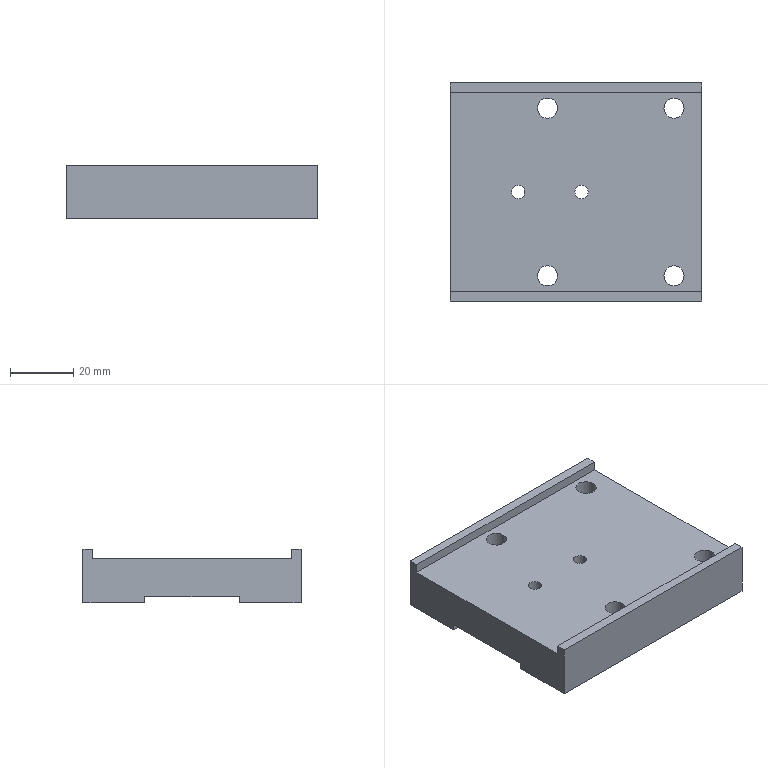Part | NX | 1 solid | 34 faces | box 79.5 x 69 x 17 mm | volume 69323 mm3 | plane 18 | cylinder 12 | cone 4 | commonest cylinder face diameters 4.2 x4 6.4 x4 11 x4
STEP:
#1=CARTESIAN_POINT('',(34.2,26.5,14.));
#2=VERTEX_POINT('',#1);
#3=CARTESIAN_POINT('',(31.,26.5,14.));
#4=DIRECTION('',(0.,0.,1.));
#5=DIRECTION('',(1.,0.,0.));
#6=AXIS2_PLACEMENT_3D('',#3,#4,#5);
#7=CIRCLE('',#6,3.2);
#8=EDGE_CURVE('',#2,#2,#7,.T.);
#9=ORIENTED_EDGE('',*,*,#8,.T.);
#10=EDGE_LOOP('',(#9));
#11=FACE_BOUND('',#10,.T.);
#12=CARTESIAN_POINT('',(27.8,26.5,6.8));
#13=VERTEX_POINT('',#12);
#14=CARTESIAN_POINT('',(31.,26.5,6.8));
#15=DIRECTION('',(0.,0.,1.));
#16=DIRECTION('',(-1.,0.,0.));
#17=AXIS2_PLACEMENT_3D('',#14,#15,#16);
#18=CIRCLE('',#17,3.2);
#19=EDGE_CURVE('',#13,#13,#18,.T.);
#20=ORIENTED_EDGE('',*,*,#19,.F.);
#21=EDGE_LOOP('',(#20));
#22=FACE_BOUND('',#21,.T.);
#23=CARTESIAN_POINT('',(31.,26.5,20.));
#24=DIRECTION('',(0.,0.,-1.));
#25=DIRECTION('',(1.,0.,0.));
#26=AXIS2_PLACEMENT_3D('',#23,#24,#25);
#27=CYLINDRICAL_SURFACE('',#26,3.2);
#28=ADVANCED_FACE('',(#11,#22),#27,.F.);
#29=CARTESIAN_POINT('',(-5.8,26.5,14.));
#30=VERTEX_POINT('',#29);
#31=CARTESIAN_POINT('',(-9.,26.5,14.));
#32=DIRECTION('',(0.,0.,1.));
#33=DIRECTION('',(1.,0.,0.));
#34=AXIS2_PLACEMENT_3D('',#31,#32,#33);
#35=CIRCLE('',#34,3.2);
#36=EDGE_CURVE('',#30,#30,#35,.T.);
#37=ORIENTED_EDGE('',*,*,#36,.T.);
#38=EDGE_LOOP('',(#37));
#39=FACE_BOUND('',#38,.T.);
#40=CARTESIAN_POINT('',(-12.2,26.5,6.8));
#41=VERTEX_POINT('',#40);
#42=CARTESIAN_POINT('',(-9.,26.5,6.8));
#43=DIRECTION('',(0.,0.,1.));
#44=DIRECTION('',(-1.,0.,0.));
#45=AXIS2_PLACEMENT_3D('',#42,#43,#44);
#46=CIRCLE('',#45,3.2);
#47=EDGE_CURVE('',#41,#41,#46,.T.);
#48=ORIENTED_EDGE('',*,*,#47,.F.);
#49=EDGE_LOOP('',(#48));
#50=FACE_BOUND('',#49,.T.);
#51=CARTESIAN_POINT('',(-9.,26.5,20.));
#52=DIRECTION('',(0.,0.,-1.));
#53=DIRECTION('',(1.,0.,0.));
#54=AXIS2_PLACEMENT_3D('',#51,#52,#53);
#55=CYLINDRICAL_SURFACE('',#54,3.2);
#56=ADVANCED_FACE('',(#39,#50),#55,.F.);
#57=CARTESIAN_POINT('',(-5.8,-26.5,14.));
#58=VERTEX_POINT('',#57);
#59=CARTESIAN_POINT('',(-9.,-26.5,14.));
#60=DIRECTION('',(0.,0.,1.));
#61=DIRECTION('',(1.,0.,0.));
#62=AXIS2_PLACEMENT_3D('',#59,#60,#61);
#63=CIRCLE('',#62,3.2);
#64=EDGE_CURVE('',#58,#58,#63,.T.);
#65=ORIENTED_EDGE('',*,*,#64,.T.);
#66=EDGE_LOOP('',(#65));
#67=FACE_BOUND('',#66,.T.);
#68=CARTESIAN_POINT('',(-12.2,-26.5,6.8));
#69=VERTEX_POINT('',#68);
#70=CARTESIAN_POINT('',(-9.,-26.5,6.8));
#71=DIRECTION('',(0.,0.,1.));
#72=DIRECTION('',(-1.,0.,0.));
#73=AXIS2_PLACEMENT_3D('',#70,#71,#72);
#74=CIRCLE('',#73,3.2);
#75=EDGE_CURVE('',#69,#69,#74,.T.);
#76=ORIENTED_EDGE('',*,*,#75,.F.);
#77=EDGE_LOOP('',(#76));
#78=FACE_BOUND('',#77,.T.);
#79=CARTESIAN_POINT('',(-9.,-26.5,20.));
#80=DIRECTION('',(0.,0.,-1.));
#81=DIRECTION('',(1.,0.,0.));
#82=AXIS2_PLACEMENT_3D('',#79,#80,#81);
#83=CYLINDRICAL_SURFACE('',#82,3.2);
#84=ADVANCED_FACE('',(#67,#78),#83,.F.);
#85=CARTESIAN_POINT('',(34.2,-26.5,14.));
#86=VERTEX_POINT('',#85);
#87=CARTESIAN_POINT('',(31.,-26.5,14.));
#88=DIRECTION('',(0.,0.,1.));
#89=DIRECTION('',(1.,0.,0.));
#90=AXIS2_PLACEMENT_3D('',#87,#88,#89);
#91=CIRCLE('',#90,3.2);
#92=EDGE_CURVE('',#86,#86,#91,.T.);
#93=ORIENTED_EDGE('',*,*,#92,.T.);
#94=EDGE_LOOP('',(#93));
#95=FACE_BOUND('',#94,.T.);
#96=CARTESIAN_POINT('',(27.8,-26.5,6.8));
#97=VERTEX_POINT('',#96);
#98=CARTESIAN_POINT('',(31.,-26.5,6.8));
#99=DIRECTION('',(0.,0.,1.));
#100=DIRECTION('',(-1.,0.,0.));
#101=AXIS2_PLACEMENT_3D('',#98,#99,#100);
#102=CIRCLE('',#101,3.2);
#103=EDGE_CURVE('',#97,#97,#102,.T.);
#104=ORIENTED_EDGE('',*,*,#103,.F.);
#105=EDGE_LOOP('',(#104));
#106=FACE_BOUND('',#105,.T.);
#107=CARTESIAN_POINT('',(31.,-26.5,20.));
#108=DIRECTION('',(0.,0.,-1.));
#109=DIRECTION('',(1.,0.,0.));
#110=AXIS2_PLACEMENT_3D('',#107,#108,#109);
#111=CYLINDRICAL_SURFACE('',#110,3.2);
#112=ADVANCED_FACE('',(#95,#106),#111,.F.);
#113=CARTESIAN_POINT('',(-16.15,0.,14.));
#114=VERTEX_POINT('',#113);
#115=CARTESIAN_POINT('',(-18.25,0.,14.));
#116=DIRECTION('',(0.,0.,-1.));
#117=DIRECTION('',(1.,0.,0.));
#118=AXIS2_PLACEMENT_3D('',#115,#116,#117);
#119=CIRCLE('',#118,2.1);
#120=EDGE_CURVE('',#114,#114,#119,.T.);
#121=ORIENTED_EDGE('',*,*,#120,.T.);
#122=EDGE_LOOP('',(#121));
#123=FACE_BOUND('',#122,.T.);
#124=CARTESIAN_POINT('',(3.85,0.,14.));
#125=VERTEX_POINT('',#124);
#126=CARTESIAN_POINT('',(1.75,0.,14.));
#127=DIRECTION('',(0.,0.,-1.));
#128=DIRECTION('',(1.,0.,0.));
#129=AXIS2_PLACEMENT_3D('',#126,#127,#128);
#130=CIRCLE('',#129,2.1);
#131=EDGE_CURVE('',#125,#125,#130,.T.);
#132=ORIENTED_EDGE('',*,*,#131,.T.);
#133=EDGE_LOOP('',(#132));
#134=FACE_BOUND('',#133,.T.);
#135=CARTESIAN_POINT('',(39.75,31.5,14.));
#136=VERTEX_POINT('',#135);
#137=CARTESIAN_POINT('',(39.75,-31.5,14.));
#138=VERTEX_POINT('',#137);
#139=CARTESIAN_POINT('',(39.75,31.5,14.));
#140=DIRECTION('',(0.,-1.,0.));
#141=VECTOR('',#140,1.);
#142=LINE('',#139,#141);
#143=EDGE_CURVE('',#136,#138,#142,.T.);
#144=ORIENTED_EDGE('',*,*,#143,.F.);
#145=CARTESIAN_POINT('',(-39.75,31.5,14.));
#146=VERTEX_POINT('',#145);
#147=CARTESIAN_POINT('',(-39.75,31.5,14.));
#148=DIRECTION('',(1.,0.,0.));
#149=VECTOR('',#148,1.);
#150=LINE('',#147,#149);
#151=EDGE_CURVE('',#146,#136,#150,.T.);
#152=ORIENTED_EDGE('',*,*,#151,.F.);
#153=CARTESIAN_POINT('',(-39.75,-31.5,14.));
#154=VERTEX_POINT('',#153);
#155=CARTESIAN_POINT('',(-39.75,31.5,14.));
#156=DIRECTION('',(0.,1.,0.));
#157=VECTOR('',#156,1.);
#158=LINE('',#155,#157);
#159=EDGE_CURVE('',#154,#146,#158,.T.);
#160=ORIENTED_EDGE('',*,*,#159,.F.);
#161=CARTESIAN_POINT('',(-39.75,-31.5,14.));
#162=DIRECTION('',(1.,0.,0.));
#163=VECTOR('',#162,1.);
#164=LINE('',#161,#163);
#165=EDGE_CURVE('',#154,#138,#164,.T.);
#166=ORIENTED_EDGE('',*,*,#165,.T.);
#167=EDGE_LOOP('',(#144,#152,#160,#166));
#168=FACE_BOUND('',#167,.T.);
#169=ORIENTED_EDGE('',*,*,#8,.F.);
#170=EDGE_LOOP('',(#169));
#171=FACE_BOUND('',#170,.T.);
#172=ORIENTED_EDGE('',*,*,#64,.F.);
#173=EDGE_LOOP('',(#172));
#174=FACE_BOUND('',#173,.T.);
#175=ORIENTED_EDGE('',*,*,#36,.F.);
#176=EDGE_LOOP('',(#175));
#177=FACE_BOUND('',#176,.T.);
#178=ORIENTED_EDGE('',*,*,#92,.F.);
#179=EDGE_LOOP('',(#178));
#180=FACE_BOUND('',#179,.T.);
#181=CARTESIAN_POINT('',(-39.75,31.5,14.));
#182=DIRECTION('',(0.,0.,1.));
#183=DIRECTION('',(-1.,0.,0.));
#184=AXIS2_PLACEMENT_3D('',#181,#182,#183);
#185=PLANE('',#184);
#186=ADVANCED_FACE('',(#123,#134,#168,#171,#174,#177,#180),#185,.T.);
#187=CARTESIAN_POINT('',(39.75,34.5,0.));
#188=VERTEX_POINT('',#187);
#189=CARTESIAN_POINT('',(39.75,34.5,17.));
#190=VERTEX_POINT('',#189);
#191=CARTESIAN_POINT('',(39.75,34.5,0.));
#192=DIRECTION('',(0.,0.,1.));
#193=VECTOR('',#192,1.);
#194=LINE('',#191,#193);
#195=EDGE_CURVE('',#188,#190,#194,.T.);
#196=ORIENTED_EDGE('',*,*,#195,.F.);
#197=CARTESIAN_POINT('',(-39.75,34.5,0.));
#198=VERTEX_POINT('',#197);
#199=CARTESIAN_POINT('',(-39.75,34.5,0.));
#200=DIRECTION('',(1.,0.,0.));
#201=VECTOR('',#200,1.);
#202=LINE('',#199,#201);
#203=EDGE_CURVE('',#198,#188,#202,.T.);
#204=ORIENTED_EDGE('',*,*,#203,.F.);
#205=CARTESIAN_POINT('',(-39.75,34.5,17.));
#206=VERTEX_POINT('',#205);
#207=CARTESIAN_POINT('',(-39.75,34.5,0.));
#208=DIRECTION('',(0.,0.,-1.));
#209=VECTOR('',#208,1.);
#210=LINE('',#207,#209);
#211=EDGE_CURVE('',#206,#198,#210,.T.);
#212=ORIENTED_EDGE('',*,*,#211,.F.);
#213=CARTESIAN_POINT('',(-39.75,34.5,17.));
#214=DIRECTION('',(1.,0.,0.));
#215=VECTOR('',#214,1.);
#216=LINE('',#213,#215);
#217=EDGE_CURVE('',#206,#190,#216,.T.);
#218=ORIENTED_EDGE('',*,*,#217,.T.);
#219=EDGE_LOOP('',(#196,#204,#212,#218));
#220=FACE_OUTER_BOUND('',#219,.T.);
#221=CARTESIAN_POINT('',(-39.75,34.5,0.));
#222=DIRECTION('',(0.,1.,0.));
#223=DIRECTION('',(0.,0.,-1.));
#224=AXIS2_PLACEMENT_3D('',#221,#222,#223);
#225=PLANE('',#224);
#226=ADVANCED_FACE('',(#220),#225,.T.);
#227=CARTESIAN_POINT('',(39.75,31.5,17.));
#228=VERTEX_POINT('',#227);
#229=CARTESIAN_POINT('',(39.75,34.5,17.));
#230=DIRECTION('',(0.,-1.,0.));
#231=VECTOR('',#230,1.);
#232=LINE('',#229,#231);
#233=EDGE_CURVE('',#190,#228,#232,.T.);
#234=ORIENTED_EDGE('',*,*,#233,.F.);
#235=ORIENTED_EDGE('',*,*,#217,.F.);
#236=CARTESIAN_POINT('',(-39.75,31.5,17.));
#237=VERTEX_POINT('',#236);
#238=CARTESIAN_POINT('',(-39.75,34.5,17.));
#239=DIRECTION('',(0.,1.,0.));
#240=VECTOR('',#239,1.);
#241=LINE('',#238,#240);
#242=EDGE_CURVE('',#237,#206,#241,.T.);
#243=ORIENTED_EDGE('',*,*,#242,.F.);
#244=CARTESIAN_POINT('',(-39.75,31.5,17.));
#245=DIRECTION('',(1.,0.,0.));
#246=VECTOR('',#245,1.);
#247=LINE('',#244,#246);
#248=EDGE_CURVE('',#237,#228,#247,.T.);
#249=ORIENTED_EDGE('',*,*,#248,.T.);
#250=EDGE_LOOP('',(#234,#235,#243,#249));
#251=FACE_OUTER_BOUND('',#250,.T.);
#252=CARTESIAN_POINT('',(-39.75,34.5,17.));
#253=DIRECTION('',(0.,0.,1.));
#254=DIRECTION('',(-1.,0.,0.));
#255=AXIS2_PLACEMENT_3D('',#252,#253,#254);
#256=PLANE('',#255);
#257=ADVANCED_FACE('',(#251),#256,.T.);
#258=CARTESIAN_POINT('',(39.75,31.5,17.));
#259=DIRECTION('',(0.,0.,-1.));
#260=VECTOR('',#259,1.);
#261=LINE('',#258,#260);
#262=EDGE_CURVE('',#228,#136,#261,.T.);
#263=ORIENTED_EDGE('',*,*,#262,.F.);
#264=ORIENTED_EDGE('',*,*,#248,.F.);
#265=CARTESIAN_POINT('',(-39.75,31.5,17.));
#266=DIRECTION('',(0.,0.,1.));
#267=VECTOR('',#266,1.);
#268=LINE('',#265,#267);
#269=EDGE_CURVE('',#146,#237,#268,.T.);
#270=ORIENTED_EDGE('',*,*,#269,.F.);
#271=ORIENTED_EDGE('',*,*,#151,.T.);
#272=EDGE_LOOP('',(#263,#264,#270,#271));
#273=FACE_OUTER_BOUND('',#272,.T.);
#274=CARTESIAN_POINT('',(-39.75,31.5,17.));
#275=DIRECTION('',(0.,-1.,0.));
#276=DIRECTION('',(0.,0.,1.));
#277=AXIS2_PLACEMENT_3D('',#274,#275,#276);
#278=PLANE('',#277);
#279=ADVANCED_FACE('',(#273),#278,.T.);
#280=CARTESIAN_POINT('',(39.75,-31.5,17.));
#281=VERTEX_POINT('',#280);
#282=CARTESIAN_POINT('',(39.75,-31.5,14.));
#283=DIRECTION('',(0.,0.,1.));
#284=VECTOR('',#283,1.);
#285=LINE('',#282,#284);
#286=EDGE_CURVE('',#138,#281,#285,.T.);
#287=ORIENTED_EDGE('',*,*,#286,.F.);
#288=ORIENTED_EDGE('',*,*,#165,.F.);
#289=CARTESIAN_POINT('',(-39.75,-31.5,17.));
#290=VERTEX_POINT('',#289);
#291=CARTESIAN_POINT('',(-39.75,-31.5,14.));
#292=DIRECTION('',(0.,0.,-1.));
#293=VECTOR('',#292,1.);
#294=LINE('',#291,#293);
#295=EDGE_CURVE('',#290,#154,#294,.T.);
#296=ORIENTED_EDGE('',*,*,#295,.F.);
#297=CARTESIAN_POINT('',(-39.75,-31.5,17.));
#298=DIRECTION('',(1.,0.,0.));
#299=VECTOR('',#298,1.);
#300=LINE('',#297,#299);
#301=EDGE_CURVE('',#290,#281,#300,.T.);
#302=ORIENTED_EDGE('',*,*,#301,.T.);
#303=EDGE_LOOP('',(#287,#288,#296,#302));
#304=FACE_OUTER_BOUND('',#303,.T.);
#305=CARTESIAN_POINT('',(-39.75,-31.5,14.));
#306=DIRECTION('',(0.,1.,0.));
#307=DIRECTION('',(0.,0.,-1.));
#308=AXIS2_PLACEMENT_3D('',#305,#306,#307);
#309=PLANE('',#308);
#310=ADVANCED_FACE('',(#304),#309,.T.);
#311=CARTESIAN_POINT('',(39.75,-34.5,17.));
#312=VERTEX_POINT('',#311);
#313=CARTESIAN_POINT('',(39.75,-31.5,17.));
#314=DIRECTION('',(0.,-1.,0.));
#315=VECTOR('',#314,1.);
#316=LINE('',#313,#315);
#317=EDGE_CURVE('',#281,#312,#316,.T.);
#318=ORIENTED_EDGE('',*,*,#317,.F.);
#319=ORIENTED_EDGE('',*,*,#301,.F.);
#320=CARTESIAN_POINT('',(-39.75,-34.5,17.));
#321=VERTEX_POINT('',#320);
#322=CARTESIAN_POINT('',(-39.75,-31.5,17.));
#323=DIRECTION('',(0.,1.,0.));
#324=VECTOR('',#323,1.);
#325=LINE('',#322,#324);
#326=EDGE_CURVE('',#321,#290,#325,.T.);
#327=ORIENTED_EDGE('',*,*,#326,.F.);
#328=CARTESIAN_POINT('',(-39.75,-34.5,17.));
#329=DIRECTION('',(1.,0.,0.));
#330=VECTOR('',#329,1.);
#331=LINE('',#328,#330);
#332=EDGE_CURVE('',#321,#312,#331,.T.);
#333=ORIENTED_EDGE('',*,*,#332,.T.);
#334=EDGE_LOOP('',(#318,#319,#327,#333));
#335=FACE_OUTER_BOUND('',#334,.T.);
#336=CARTESIAN_POINT('',(-39.75,-31.5,17.));
#337=DIRECTION('',(0.,0.,1.));
#338=DIRECTION('',(-1.,0.,0.));
#339=AXIS2_PLACEMENT_3D('',#336,#337,#338);
#340=PLANE('',#339);
#341=ADVANCED_FACE('',(#335),#340,.T.);
#342=CARTESIAN_POINT('',(39.75,-34.5,0.));
#343=VERTEX_POINT('',#342);
#344=CARTESIAN_POINT('',(39.75,-34.5,17.));
#345=DIRECTION('',(0.,0.,-1.));
#346=VECTOR('',#345,1.);
#347=LINE('',#344,#346);
#348=EDGE_CURVE('',#312,#343,#347,.T.);
#349=ORIENTED_EDGE('',*,*,#348,.F.);
#350=ORIENTED_EDGE('',*,*,#332,.F.);
#351=CARTESIAN_POINT('',(-39.75,-34.5,0.));
#352=VERTEX_POINT('',#351);
#353=CARTESIAN_POINT('',(-39.75,-34.5,17.));
#354=DIRECTION('',(0.,0.,1.));
#355=VECTOR('',#354,1.);
#356=LINE('',#353,#355);
#357=EDGE_CURVE('',#352,#321,#356,.T.);
#358=ORIENTED_EDGE('',*,*,#357,.F.);
#359=CARTESIAN_POINT('',(-39.75,-34.5,0.));
#360=DIRECTION('',(1.,0.,0.));
#361=VECTOR('',#360,1.);
#362=LINE('',#359,#361);
#363=EDGE_CURVE('',#352,#343,#362,.T.);
#364=ORIENTED_EDGE('',*,*,#363,.T.);
#365=EDGE_LOOP('',(#349,#350,#358,#364));
#366=FACE_OUTER_BOUND('',#365,.T.);
#367=CARTESIAN_POINT('',(-39.75,-34.5,17.));
#368=DIRECTION('',(0.,-1.,0.));
#369=DIRECTION('',(0.,0.,1.));
#370=AXIS2_PLACEMENT_3D('',#367,#368,#369);
#371=PLANE('',#370);
#372=ADVANCED_FACE('',(#366),#371,.T.);
#373=CARTESIAN_POINT('',(25.5,-26.5,0.));
#374=VERTEX_POINT('',#373);
#375=CARTESIAN_POINT('',(31.,-26.5,0.));
#376=DIRECTION('',(0.,0.,-1.));
#377=DIRECTION('',(-1.,0.,0.));
#378=AXIS2_PLACEMENT_3D('',#375,#376,#377);
#379=CIRCLE('',#378,5.5);
#380=EDGE_CURVE('',#374,#374,#379,.T.);
#381=ORIENTED_EDGE('',*,*,#380,.F.);
#382=EDGE_LOOP('',(#381));
#383=FACE_BOUND('',#382,.T.);
#384=CARTESIAN_POINT('',(-14.5,-26.5,0.));
#385=VERTEX_POINT('',#384);
#386=CARTESIAN_POINT('',(-9.,-26.5,0.));
#387=DIRECTION('',(0.,0.,-1.));
#388=DIRECTION('',(-1.,0.,0.));
#389=AXIS2_PLACEMENT_3D('',#386,#387,#388);
#390=CIRCLE('',#389,5.5);
#391=EDGE_CURVE('',#385,#385,#390,.T.);
#392=ORIENTED_EDGE('',*,*,#391,.F.);
#393=EDGE_LOOP('',(#392));
#394=FACE_BOUND('',#393,.T.);
#395=CARTESIAN_POINT('',(39.75,-15.,0.));
#396=VERTEX_POINT('',#395);
#397=CARTESIAN_POINT('',(39.75,-34.5,0.));
#398=DIRECTION('',(0.,1.,0.));
#399=VECTOR('',#398,1.);
#400=LINE('',#397,#399);
#401=EDGE_CURVE('',#343,#396,#400,.T.);
#402=ORIENTED_EDGE('',*,*,#401,.F.);
#403=ORIENTED_EDGE('',*,*,#363,.F.);
#404=CARTESIAN_POINT('',(-39.75,-15.,0.));
#405=VERTEX_POINT('',#404);
#406=CARTESIAN_POINT('',(-39.75,-34.5,0.));
#407=DIRECTION('',(0.,-1.,0.));
#408=VECTOR('',#407,1.);
#409=LINE('',#406,#408);
#410=EDGE_CURVE('',#405,#352,#409,.T.);
#411=ORIENTED_EDGE('',*,*,#410,.F.);
#412=CARTESIAN_POINT('',(-39.75,-15.,0.));
#413=DIRECTION('',(1.,0.,0.));
#414=VECTOR('',#413,1.);
#415=LINE('',#412,#414);
#416=EDGE_CURVE('',#405,#396,#415,.T.);
#417=ORIENTED_EDGE('',*,*,#416,.T.);
#418=EDGE_LOOP('',(#402,#403,#411,#417));
#419=FACE_BOUND('',#418,.T.);
#420=CARTESIAN_POINT('',(-39.75,-34.5,0.));
#421=DIRECTION('',(0.,0.,-1.));
#422=DIRECTION('',(1.,0.,0.));
#423=AXIS2_PLACEMENT_3D('',#420,#421,#422);
#424=PLANE('',#423);
#425=ADVANCED_FACE('',(#383,#394,#419),#424,.T.);
#426=CARTESIAN_POINT('',(39.75,-15.,2.));
#427=VERTEX_POINT('',#426);
#428=CARTESIAN_POINT('',(39.75,-15.,0.));
#429=DIRECTION('',(0.,0.,1.));
#430=VECTOR('',#429,1.);
#431=LINE('',#428,#430);
#432=EDGE_CURVE('',#396,#427,#431,.T.);
#433=ORIENTED_EDGE('',*,*,#432,.F.);
#434=ORIENTED_EDGE('',*,*,#416,.F.);
#435=CARTESIAN_POINT('',(-39.75,-15.,2.));
#436=VERTEX_POINT('',#435);
#437=CARTESIAN_POINT('',(-39.75,-15.,0.));
#438=DIRECTION('',(0.,0.,-1.));
#439=VECTOR('',#438,1.);
#440=LINE('',#437,#439);
#441=EDGE_CURVE('',#436,#405,#440,.T.);
#442=ORIENTED_EDGE('',*,*,#441,.F.);
#443=CARTESIAN_POINT('',(-39.75,-15.,2.));
#444=DIRECTION('',(1.,0.,0.));
#445=VECTOR('',#444,1.);
#446=LINE('',#443,#445);
#447=EDGE_CURVE('',#436,#427,#446,.T.);
#448=ORIENTED_EDGE('',*,*,#447,.T.);
#449=EDGE_LOOP('',(#433,#434,#442,#448));
#450=FACE_OUTER_BOUND('',#449,.T.);
#451=CARTESIAN_POINT('',(-39.75,-15.,0.));
#452=DIRECTION('',(0.,1.,0.));
#453=DIRECTION('',(0.,0.,-1.));
#454=AXIS2_PLACEMENT_3D('',#451,#452,#453);
#455=PLANE('',#454);
#456=ADVANCED_FACE('',(#450),#455,.T.);
#457=CARTESIAN_POINT('',(-20.35,0.,2.));
#458=VERTEX_POINT('',#457);
#459=CARTESIAN_POINT('',(-18.25,0.,2.));
#460=DIRECTION('',(0.,0.,1.));
#461=DIRECTION('',(-1.,0.,0.));
#462=AXIS2_PLACEMENT_3D('',#459,#460,#461);
#463=CIRCLE('',#462,2.1);
#464=EDGE_CURVE('',#458,#458,#463,.T.);
#465=ORIENTED_EDGE('',*,*,#464,.T.);
#466=EDGE_LOOP('',(#465));
#467=FACE_BOUND('',#466,.T.);
#468=CARTESIAN_POINT('',(-0.35,0.,2.));
#469=VERTEX_POINT('',#468);
#470=CARTESIAN_POINT('',(1.75,0.,2.));
#471=DIRECTION('',(0.,0.,1.));
#472=DIRECTION('',(-1.,0.,0.));
#473=AXIS2_PLACEMENT_3D('',#470,#471,#472);
#474=CIRCLE('',#473,2.1);
#475=EDGE_CURVE('',#469,#469,#474,.T.);
#476=ORIENTED_EDGE('',*,*,#475,.T.);
#477=EDGE_LOOP('',(#476));
#478=FACE_BOUND('',#477,.T.);
#479=CARTESIAN_POINT('',(39.75,15.,2.));
#480=VERTEX_POINT('',#479);
#481=CARTESIAN_POINT('',(39.75,-15.,2.));
#482=DIRECTION('',(0.,1.,0.));
#483=VECTOR('',#482,1.);
#484=LINE('',#481,#483);
#485=EDGE_CURVE('',#427,#480,#484,.T.);
#486=ORIENTED_EDGE('',*,*,#485,.F.);
#487=ORIENTED_EDGE('',*,*,#447,.F.);
#488=CARTESIAN_POINT('',(-39.75,15.,2.));
#489=VERTEX_POINT('',#488);
#490=CARTESIAN_POINT('',(-39.75,-15.,2.));
#491=DIRECTION('',(0.,-1.,0.));
#492=VECTOR('',#491,1.);
#493=LINE('',#490,#492);
#494=EDGE_CURVE('',#489,#436,#493,.T.);
#495=ORIENTED_EDGE('',*,*,#494,.F.);
#496=CARTESIAN_POINT('',(-39.75,15.,2.));
#497=DIRECTION('',(1.,0.,0.));
#498=VECTOR('',#497,1.);
#499=LINE('',#496,#498);
#500=EDGE_CURVE('',#489,#480,#499,.T.);
#501=ORIENTED_EDGE('',*,*,#500,.T.);
#502=EDGE_LOOP('',(#486,#487,#495,#501));
#503=FACE_BOUND('',#502,.T.);
#504=CARTESIAN_POINT('',(-39.75,-15.,2.));
#505=DIRECTION('',(0.,0.,-1.));
#506=DIRECTION('',(1.,0.,0.));
#507=AXIS2_PLACEMENT_3D('',#504,#505,#506);
#508=PLANE('',#507);
#509=ADVANCED_FACE('',(#467,#478,#503),#508,.T.);
#510=CARTESIAN_POINT('',(39.75,15.,0.));
#511=VERTEX_POINT('',#510);
#512=CARTESIAN_POINT('',(39.75,15.,2.));
#513=DIRECTION('',(0.,0.,-1.));
#514=VECTOR('',#513,1.);
#515=LINE('',#512,#514);
#516=EDGE_CURVE('',#480,#511,#515,.T.);
#517=ORIENTED_EDGE('',*,*,#516,.F.);
#518=ORIENTED_EDGE('',*,*,#500,.F.);
#519=CARTESIAN_POINT('',(-39.75,15.,0.));
#520=VERTEX_POINT('',#519);
#521=CARTESIAN_POINT('',(-39.75,15.,2.));
#522=DIRECTION('',(0.,0.,1.));
#523=VECTOR('',#522,1.);
#524=LINE('',#521,#523);
#525=EDGE_CURVE('',#520,#489,#524,.T.);
#526=ORIENTED_EDGE('',*,*,#525,.F.);
#527=CARTESIAN_POINT('',(-39.75,15.,0.));
#528=DIRECTION('',(1.,0.,0.));
#529=VECTOR('',#528,1.);
#530=LINE('',#527,#529);
#531=EDGE_CURVE('',#520,#511,#530,.T.);
#532=ORIENTED_EDGE('',*,*,#531,.T.);
#533=EDGE_LOOP('',(#517,#518,#526,#532));
#534=FACE_OUTER_BOUND('',#533,.T.);
#535=CARTESIAN_POINT('',(-39.75,15.,2.));
#536=DIRECTION('',(0.,-1.,0.));
#537=DIRECTION('',(0.,0.,1.));
#538=AXIS2_PLACEMENT_3D('',#535,#536,#537);
#539=PLANE('',#538);
#540=ADVANCED_FACE('',(#534),#539,.T.);
#541=CARTESIAN_POINT('',(-14.5,26.5,0.));
#542=VERTEX_POINT('',#541);
#543=CARTESIAN_POINT('',(-9.,26.5,0.));
#544=DIRECTION('',(0.,0.,-1.));
#545=DIRECTION('',(-1.,0.,0.));
#546=AXIS2_PLACEMENT_3D('',#543,#544,#545);
#547=CIRCLE('',#546,5.5);
#548=EDGE_CURVE('',#542,#542,#547,.T.);
#549=ORIENTED_EDGE('',*,*,#548,.F.);
#550=EDGE_LOOP('',(#549));
#551=FACE_BOUND('',#550,.T.);
#552=CARTESIAN_POINT('',(25.5,26.5,0.));
#553=VERTEX_POINT('',#552);
#554=CARTESIAN_POINT('',(31.,26.5,0.));
#555=DIRECTION('',(0.,0.,-1.));
#556=DIRECTION('',(-1.,0.,0.));
#557=AXIS2_PLACEMENT_3D('',#554,#555,#556);
#558=CIRCLE('',#557,5.5);
#559=EDGE_CURVE('',#553,#553,#558,.T.);
#560=ORIENTED_EDGE('',*,*,#559,.F.);
#561=EDGE_LOOP('',(#560));
#562=FACE_BOUND('',#561,.T.);
#563=CARTESIAN_POINT('',(39.75,15.,0.));
#564=DIRECTION('',(0.,1.,0.));
#565=VECTOR('',#564,1.);
#566=LINE('',#563,#565);
#567=EDGE_CURVE('',#511,#188,#566,.T.);
#568=ORIENTED_EDGE('',*,*,#567,.F.);
#569=ORIENTED_EDGE('',*,*,#531,.F.);
#570=CARTESIAN_POINT('',(-39.75,15.,0.));
#571=DIRECTION('',(0.,-1.,0.));
#572=VECTOR('',#571,1.);
#573=LINE('',#570,#572);
#574=EDGE_CURVE('',#198,#520,#573,.T.);
#575=ORIENTED_EDGE('',*,*,#574,.F.);
#576=ORIENTED_EDGE('',*,*,#203,.T.);
#577=EDGE_LOOP('',(#568,#569,#575,#576));
#578=FACE_BOUND('',#577,.T.);
#579=CARTESIAN_POINT('',(-39.75,15.,0.));
#580=DIRECTION('',(0.,0.,-1.));
#581=DIRECTION('',(1.,0.,0.));
#582=AXIS2_PLACEMENT_3D('',#579,#580,#581);
#583=PLANE('',#582);
#584=ADVANCED_FACE('',(#551,#562,#578),#583,.T.);
#585=ORIENTED_EDGE('',*,*,#211,.T.);
#586=ORIENTED_EDGE('',*,*,#574,.T.);
#587=ORIENTED_EDGE('',*,*,#525,.T.);
#588=ORIENTED_EDGE('',*,*,#494,.T.);
#589=ORIENTED_EDGE('',*,*,#441,.T.);
#590=ORIENTED_EDGE('',*,*,#410,.T.);
#591=ORIENTED_EDGE('',*,*,#357,.T.);
#592=ORIENTED_EDGE('',*,*,#326,.T.);
#593=ORIENTED_EDGE('',*,*,#295,.T.);
#594=ORIENTED_EDGE('',*,*,#159,.T.);
#595=ORIENTED_EDGE('',*,*,#269,.T.);
#596=ORIENTED_EDGE('',*,*,#242,.T.);
#597=EDGE_LOOP('',(#585,#586,#587,#588,#589,#590,#591,#592,#593,#594,#595,#596));
#598=FACE_OUTER_BOUND('',#597,.T.);
#599=CARTESIAN_POINT('',(-39.75,0.,0.));
#600=DIRECTION('',(1.,0.,0.));
#601=DIRECTION('',(0.,0.,1.));
#602=AXIS2_PLACEMENT_3D('',#599,#600,#601);
#603=PLANE('',#602);
#604=ADVANCED_FACE('',(#598),#603,.F.);
#605=CARTESIAN_POINT('',(39.75,18.,5.5));
#606=VERTEX_POINT('',#605);
#607=CARTESIAN_POINT('',(39.75,18.,8.));
#608=DIRECTION('',(-1.,0.,0.));
#609=DIRECTION('',(0.,0.,-1.));
#610=AXIS2_PLACEMENT_3D('',#607,#608,#609);
#611=CIRCLE('',#610,2.5);
#612=EDGE_CURVE('',#606,#606,#611,.T.);
#613=ORIENTED_EDGE('',*,*,#612,.T.);
#614=EDGE_LOOP('',(#613));
#615=FACE_BOUND('',#614,.T.);
#616=CARTESIAN_POINT('',(39.75,-18.,5.5));
#617=VERTEX_POINT('',#616);
#618=CARTESIAN_POINT('',(39.75,-18.,8.));
#619=DIRECTION('',(-1.,0.,0.));
#620=DIRECTION('',(0.,0.,-1.));
#621=AXIS2_PLACEMENT_3D('',#618,#619,#620);
#622=CIRCLE('',#621,2.5);
#623=EDGE_CURVE('',#617,#617,#622,.T.);
#624=ORIENTED_EDGE('',*,*,#623,.T.);
#625=EDGE_LOOP('',(#624));
#626=FACE_BOUND('',#625,.T.);
#627=ORIENTED_EDGE('',*,*,#195,.T.);
#628=ORIENTED_EDGE('',*,*,#233,.T.);
#629=ORIENTED_EDGE('',*,*,#262,.T.);
#630=ORIENTED_EDGE('',*,*,#143,.T.);
#631=ORIENTED_EDGE('',*,*,#286,.T.);
#632=ORIENTED_EDGE('',*,*,#317,.T.);
#633=ORIENTED_EDGE('',*,*,#348,.T.);
#634=ORIENTED_EDGE('',*,*,#401,.T.);
#635=ORIENTED_EDGE('',*,*,#432,.T.);
#636=ORIENTED_EDGE('',*,*,#485,.T.);
#637=ORIENTED_EDGE('',*,*,#516,.T.);
#638=ORIENTED_EDGE('',*,*,#567,.T.);
#639=EDGE_LOOP('',(#627,#628,#629,#630,#631,#632,#633,#634,#635,#636,#637,#638));
#640=FACE_BOUND('',#639,.T.);
#641=CARTESIAN_POINT('',(39.75,0.,0.));
#642=DIRECTION('',(1.,0.,0.));
#643=DIRECTION('',(0.,0.,1.));
#644=AXIS2_PLACEMENT_3D('',#641,#642,#643);
#645=PLANE('',#644);
#646=ADVANCED_FACE('',(#615,#626,#640),#645,.T.);
#647=ORIENTED_EDGE('',*,*,#131,.F.);
#648=EDGE_LOOP('',(#647));
#649=FACE_BOUND('',#648,.T.);
#650=ORIENTED_EDGE('',*,*,#475,.F.);
#651=EDGE_LOOP('',(#650));
#652=FACE_BOUND('',#651,.T.);
#653=CARTESIAN_POINT('',(1.75,0.,20.));
#654=DIRECTION('',(0.,0.,-1.));
#655=DIRECTION('',(1.,0.,0.));
#656=AXIS2_PLACEMENT_3D('',#653,#654,#655);
#657=CYLINDRICAL_SURFACE('',#656,2.1);
#658=ADVANCED_FACE('',(#649,#652),#657,.F.);
#659=ORIENTED_EDGE('',*,*,#120,.F.);
#660=EDGE_LOOP('',(#659));
#661=FACE_BOUND('',#660,.T.);
#662=ORIENTED_EDGE('',*,*,#464,.F.);
#663=EDGE_LOOP('',(#662));
#664=FACE_BOUND('',#663,.T.);
#665=CARTESIAN_POINT('',(-18.25,0.,20.));
#666=DIRECTION('',(0.,0.,-1.));
#667=DIRECTION('',(1.,0.,0.));
#668=AXIS2_PLACEMENT_3D('',#665,#666,#667);
#669=CYLINDRICAL_SURFACE('',#668,2.1);
#670=ADVANCED_FACE('',(#661,#664),#669,.F.);
#671=CARTESIAN_POINT('',(25.5,-26.5,6.8));
#672=VERTEX_POINT('',#671);
#673=CARTESIAN_POINT('',(31.,-26.5,6.8));
#674=DIRECTION('',(0.,0.,1.));
#675=DIRECTION('',(-1.,0.,0.));
#676=AXIS2_PLACEMENT_3D('',#673,#674,#675);
#677=CIRCLE('',#676,5.5);
#678=EDGE_CURVE('',#672,#672,#677,.T.);
#679=ORIENTED_EDGE('',*,*,#678,.F.);
#680=EDGE_LOOP('',(#679));
#681=FACE_BOUND('',#680,.T.);
#682=ORIENTED_EDGE('',*,*,#103,.T.);
#683=EDGE_LOOP('',(#682));
#684=FACE_BOUND('',#683,.T.);
#685=CARTESIAN_POINT('',(31.,-26.5,6.8));
#686=DIRECTION('',(0.,0.,-1.));
#687=DIRECTION('',(1.,0.,0.));
#688=AXIS2_PLACEMENT_3D('',#685,#686,#687);
#689=PLANE('',#688);
#690=ADVANCED_FACE('',(#681,#684),#689,.T.);
#691=ORIENTED_EDGE('',*,*,#380,.T.);
#692=EDGE_LOOP('',(#691));
#693=FACE_BOUND('',#692,.T.);
#694=ORIENTED_EDGE('',*,*,#678,.T.);
#695=EDGE_LOOP('',(#694));
#696=FACE_BOUND('',#695,.T.);
#697=CARTESIAN_POINT('',(31.,-26.5,6.8));
#698=DIRECTION('',(0.,0.,-1.));
#699=DIRECTION('',(1.,0.,0.));
#700=AXIS2_PLACEMENT_3D('',#697,#698,#699);
#701=CYLINDRICAL_SURFACE('',#700,5.5);
#702=ADVANCED_FACE('',(#693,#696),#701,.F.);
#703=CARTESIAN_POINT('',(-14.5,-26.5,6.8));
#704=VERTEX_POINT('',#703);
#705=CARTESIAN_POINT('',(-9.,-26.5,6.8));
#706=DIRECTION('',(0.,0.,1.));
#707=DIRECTION('',(-1.,0.,0.));
#708=AXIS2_PLACEMENT_3D('',#705,#706,#707);
#709=CIRCLE('',#708,5.5);
#710=EDGE_CURVE('',#704,#704,#709,.T.);
#711=ORIENTED_EDGE('',*,*,#710,.F.);
#712=EDGE_LOOP('',(#711));
#713=FACE_BOUND('',#712,.T.);
#714=ORIENTED_EDGE('',*,*,#75,.T.);
#715=EDGE_LOOP('',(#714));
#716=FACE_BOUND('',#715,.T.);
#717=CARTESIAN_POINT('',(-9.,-26.5,6.8));
#718=DIRECTION('',(0.,0.,-1.));
#719=DIRECTION('',(1.,0.,0.));
#720=AXIS2_PLACEMENT_3D('',#717,#718,#719);
#721=PLANE('',#720);
#722=ADVANCED_FACE('',(#713,#716),#721,.T.);
#723=ORIENTED_EDGE('',*,*,#391,.T.);
#724=EDGE_LOOP('',(#723));
#725=FACE_BOUND('',#724,.T.);
#726=ORIENTED_EDGE('',*,*,#710,.T.);
#727=EDGE_LOOP('',(#726));
#728=FACE_BOUND('',#727,.T.);
#729=CARTESIAN_POINT('',(-9.,-26.5,6.8));
#730=DIRECTION('',(0.,0.,-1.));
#731=DIRECTION('',(1.,0.,0.));
#732=AXIS2_PLACEMENT_3D('',#729,#730,#731);
#733=CYLINDRICAL_SURFACE('',#732,5.5);
#734=ADVANCED_FACE('',(#725,#728),#733,.F.);
#735=CARTESIAN_POINT('',(-14.5,26.5,6.8));
#736=VERTEX_POINT('',#735);
#737=CARTESIAN_POINT('',(-9.,26.5,6.8));
#738=DIRECTION('',(0.,0.,1.));
#739=DIRECTION('',(-1.,0.,0.));
#740=AXIS2_PLACEMENT_3D('',#737,#738,#739);
#741=CIRCLE('',#740,5.5);
#742=EDGE_CURVE('',#736,#736,#741,.T.);
#743=ORIENTED_EDGE('',*,*,#742,.F.);
#744=EDGE_LOOP('',(#743));
#745=FACE_BOUND('',#744,.T.);
#746=ORIENTED_EDGE('',*,*,#47,.T.);
#747=EDGE_LOOP('',(#746));
#748=FACE_BOUND('',#747,.T.);
#749=CARTESIAN_POINT('',(-9.,26.5,6.8));
#750=DIRECTION('',(0.,0.,-1.));
#751=DIRECTION('',(1.,0.,0.));
#752=AXIS2_PLACEMENT_3D('',#749,#750,#751);
#753=PLANE('',#752);
#754=ADVANCED_FACE('',(#745,#748),#753,.T.);
#755=ORIENTED_EDGE('',*,*,#548,.T.);
#756=EDGE_LOOP('',(#755));
#757=FACE_BOUND('',#756,.T.);
#758=ORIENTED_EDGE('',*,*,#742,.T.);
#759=EDGE_LOOP('',(#758));
#760=FACE_BOUND('',#759,.T.);
#761=CARTESIAN_POINT('',(-9.,26.5,6.8));
#762=DIRECTION('',(0.,0.,-1.));
#763=DIRECTION('',(1.,0.,0.));
#764=AXIS2_PLACEMENT_3D('',#761,#762,#763);
#765=CYLINDRICAL_SURFACE('',#764,5.5);
#766=ADVANCED_FACE('',(#757,#760),#765,.F.);
#767=CARTESIAN_POINT('',(25.5,26.5,6.8));
#768=VERTEX_POINT('',#767);
#769=CARTESIAN_POINT('',(31.,26.5,6.8));
#770=DIRECTION('',(0.,0.,1.));
#771=DIRECTION('',(-1.,0.,0.));
#772=AXIS2_PLACEMENT_3D('',#769,#770,#771);
#773=CIRCLE('',#772,5.5);
#774=EDGE_CURVE('',#768,#768,#773,.T.);
#775=ORIENTED_EDGE('',*,*,#774,.F.);
#776=EDGE_LOOP('',(#775));
#777=FACE_BOUND('',#776,.T.);
#778=ORIENTED_EDGE('',*,*,#19,.T.);
#779=EDGE_LOOP('',(#778));
#780=FACE_BOUND('',#779,.T.);
#781=CARTESIAN_POINT('',(31.,26.5,6.8));
#782=DIRECTION('',(0.,0.,-1.));
#783=DIRECTION('',(1.,0.,0.));
#784=AXIS2_PLACEMENT_3D('',#781,#782,#783);
#785=PLANE('',#784);
#786=ADVANCED_FACE('',(#777,#780),#785,.T.);
#787=ORIENTED_EDGE('',*,*,#559,.T.);
#788=EDGE_LOOP('',(#787));
#789=FACE_BOUND('',#788,.T.);
#790=ORIENTED_EDGE('',*,*,#774,.T.);
#791=EDGE_LOOP('',(#790));
#792=FACE_BOUND('',#791,.T.);
#793=CARTESIAN_POINT('',(31.,26.5,6.8));
#794=DIRECTION('',(0.,0.,-1.));
#795=DIRECTION('',(1.,0.,0.));
#796=AXIS2_PLACEMENT_3D('',#793,#794,#795);
#797=CYLINDRICAL_SURFACE('',#796,5.5);
#798=ADVANCED_FACE('',(#789,#792),#797,.F.);
#799=CARTESIAN_POINT('',(29.75,-18.,10.1));
#800=VERTEX_POINT('',#799);
#801=CARTESIAN_POINT('',(29.75,-18.,8.));
#802=DIRECTION('',(1.,0.,0.));
#803=DIRECTION('',(0.,0.,1.));
#804=AXIS2_PLACEMENT_3D('',#801,#802,#803);
#805=CIRCLE('',#804,2.1);
#806=EDGE_CURVE('',#800,#800,#805,.T.);
#807=ORIENTED_EDGE('',*,*,#806,.T.);
#808=EDGE_LOOP('',(#807));
#809=FACE_BOUND('',#808,.T.);
#810=CARTESIAN_POINT('',(28.488,-18.,8.));
#811=VERTEX_POINT('',#810);
#812=VERTEX_LOOP('',#811);
#813=FACE_BOUND('',#812,.T.);
#814=CARTESIAN_POINT('',(29.75,-18.,8.));
#815=DIRECTION('',(1.,0.,0.));
#816=DIRECTION('',(0.,0.,1.));
#817=AXIS2_PLACEMENT_3D('',#814,#815,#816);
#818=CONICAL_SURFACE('',#817,2.1,59.);
#819=ADVANCED_FACE('',(#809,#813),#818,.F.);
#820=CARTESIAN_POINT('',(39.35,-18.,5.9));
#821=VERTEX_POINT('',#820);
#822=CARTESIAN_POINT('',(39.35,-18.,8.));
#823=DIRECTION('',(1.,0.,0.));
#824=DIRECTION('',(0.,0.,-1.));
#825=AXIS2_PLACEMENT_3D('',#822,#823,#824);
#826=CIRCLE('',#825,2.1);
#827=EDGE_CURVE('',#821,#821,#826,.T.);
#828=ORIENTED_EDGE('',*,*,#827,.T.);
#829=EDGE_LOOP('',(#828));
#830=FACE_BOUND('',#829,.T.);
#831=ORIENTED_EDGE('',*,*,#806,.F.);
#832=EDGE_LOOP('',(#831));
#833=FACE_BOUND('',#832,.T.);
#834=CARTESIAN_POINT('',(39.75,-18.,8.));
#835=DIRECTION('',(-1.,0.,0.));
#836=DIRECTION('',(0.,0.,-1.));
#837=AXIS2_PLACEMENT_3D('',#834,#835,#836);
#838=CYLINDRICAL_SURFACE('',#837,2.1);
#839=ADVANCED_FACE('',(#830,#833),#838,.F.);
#840=ORIENTED_EDGE('',*,*,#827,.F.);
#841=EDGE_LOOP('',(#840));
#842=FACE_BOUND('',#841,.T.);
#843=ORIENTED_EDGE('',*,*,#623,.F.);
#844=EDGE_LOOP('',(#843));
#845=FACE_BOUND('',#844,.T.);
#846=CARTESIAN_POINT('',(39.75,-18.,8.));
#847=DIRECTION('',(1.,0.,0.));
#848=DIRECTION('',(0.,0.,1.));
#849=AXIS2_PLACEMENT_3D('',#846,#847,#848);
#850=CONICAL_SURFACE('',#849,2.5,45.);
#851=ADVANCED_FACE('',(#842,#845),#850,.F.);
#852=CARTESIAN_POINT('',(29.75,18.,10.1));
#853=VERTEX_POINT('',#852);
#854=CARTESIAN_POINT('',(29.75,18.,8.));
#855=DIRECTION('',(1.,0.,0.));
#856=DIRECTION('',(0.,0.,1.));
#857=AXIS2_PLACEMENT_3D('',#854,#855,#856);
#858=CIRCLE('',#857,2.1);
#859=EDGE_CURVE('',#853,#853,#858,.T.);
#860=ORIENTED_EDGE('',*,*,#859,.T.);
#861=EDGE_LOOP('',(#860));
#862=FACE_BOUND('',#861,.T.);
#863=CARTESIAN_POINT('',(28.488,18.,8.));
#864=VERTEX_POINT('',#863);
#865=VERTEX_LOOP('',#864);
#866=FACE_BOUND('',#865,.T.);
#867=CARTESIAN_POINT('',(29.75,18.,8.));
#868=DIRECTION('',(1.,0.,0.));
#869=DIRECTION('',(0.,0.,1.));
#870=AXIS2_PLACEMENT_3D('',#867,#868,#869);
#871=CONICAL_SURFACE('',#870,2.1,59.);
#872=ADVANCED_FACE('',(#862,#866),#871,.F.);
#873=CARTESIAN_POINT('',(39.35,18.,5.9));
#874=VERTEX_POINT('',#873);
#875=CARTESIAN_POINT('',(39.35,18.,8.));
#876=DIRECTION('',(1.,0.,0.));
#877=DIRECTION('',(0.,0.,-1.));
#878=AXIS2_PLACEMENT_3D('',#875,#876,#877);
#879=CIRCLE('',#878,2.1);
#880=EDGE_CURVE('',#874,#874,#879,.T.);
#881=ORIENTED_EDGE('',*,*,#880,.T.);
#882=EDGE_LOOP('',(#881));
#883=FACE_BOUND('',#882,.T.);
#884=ORIENTED_EDGE('',*,*,#859,.F.);
#885=EDGE_LOOP('',(#884));
#886=FACE_BOUND('',#885,.T.);
#887=CARTESIAN_POINT('',(39.75,18.,8.));
#888=DIRECTION('',(-1.,0.,0.));
#889=DIRECTION('',(0.,0.,-1.));
#890=AXIS2_PLACEMENT_3D('',#887,#888,#889);
#891=CYLINDRICAL_SURFACE('',#890,2.1);
#892=ADVANCED_FACE('',(#883,#886),#891,.F.);
#893=ORIENTED_EDGE('',*,*,#880,.F.);
#894=EDGE_LOOP('',(#893));
#895=FACE_BOUND('',#894,.T.);
#896=ORIENTED_EDGE('',*,*,#612,.F.);
#897=EDGE_LOOP('',(#896));
#898=FACE_BOUND('',#897,.T.);
#899=CARTESIAN_POINT('',(39.75,18.,8.));
#900=DIRECTION('',(1.,0.,0.));
#901=DIRECTION('',(0.,0.,1.));
#902=AXIS2_PLACEMENT_3D('',#899,#900,#901);
#903=CONICAL_SURFACE('',#902,2.5,45.);
#904=ADVANCED_FACE('',(#895,#898),#903,.F.);
#905=CLOSED_SHELL('',(#28,#56,#84,#112,#186,#226,#257,#279,#310,#341,#372,#425,#456,#509,#540,#584,#604,#646,#658,#670,#690,#702,#722,#734,#754,#766,#786,#798,#819,#839,#851,#872,#892,#904));
#906=MANIFOLD_SOLID_BREP('',#905);
#907=(LENGTH_UNIT()NAMED_UNIT(*)SI_UNIT(.MILLI.,.METRE.));
#908=UNCERTAINTY_MEASURE_WITH_UNIT(LENGTH_MEASURE(0.00002),#907,'','');
#909=(NAMED_UNIT(*)PLANE_ANGLE_UNIT()SI_UNIT($,.RADIAN.));
#910=PLANE_ANGLE_MEASURE_WITH_UNIT(PLANE_ANGLE_MEASURE(0.01745),#909);
#911=DIMENSIONAL_EXPONENTS(0.,0.,0.,0.,0.,0.,0.);
#912=(CONVERSION_BASED_UNIT('DEGREE',#910)NAMED_UNIT(#911)PLANE_ANGLE_UNIT());
#913=(NAMED_UNIT(*)SI_UNIT($,.STERADIAN.)SOLID_ANGLE_UNIT());
#914=(GEOMETRIC_REPRESENTATION_CONTEXT(3)GLOBAL_UNCERTAINTY_ASSIGNED_CONTEXT((#908))GLOBAL_UNIT_ASSIGNED_CONTEXT((#907,#912,#913))REPRESENTATION_CONTEXT('',''));
#915=ADVANCED_BREP_SHAPE_REPRESENTATION('',(#906),#914);